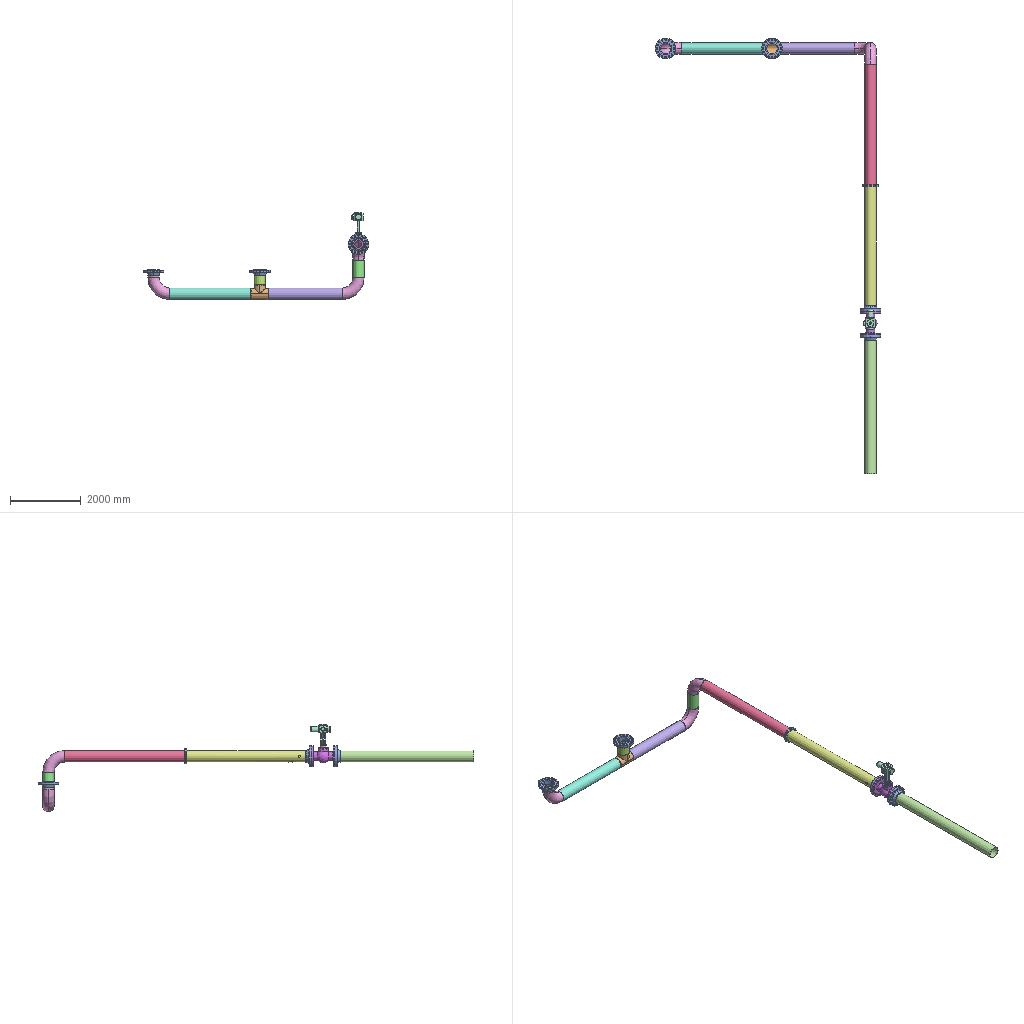Assembly | NX | 16 different items | 22 placed | box 6356 x 12301 x 2462 mm
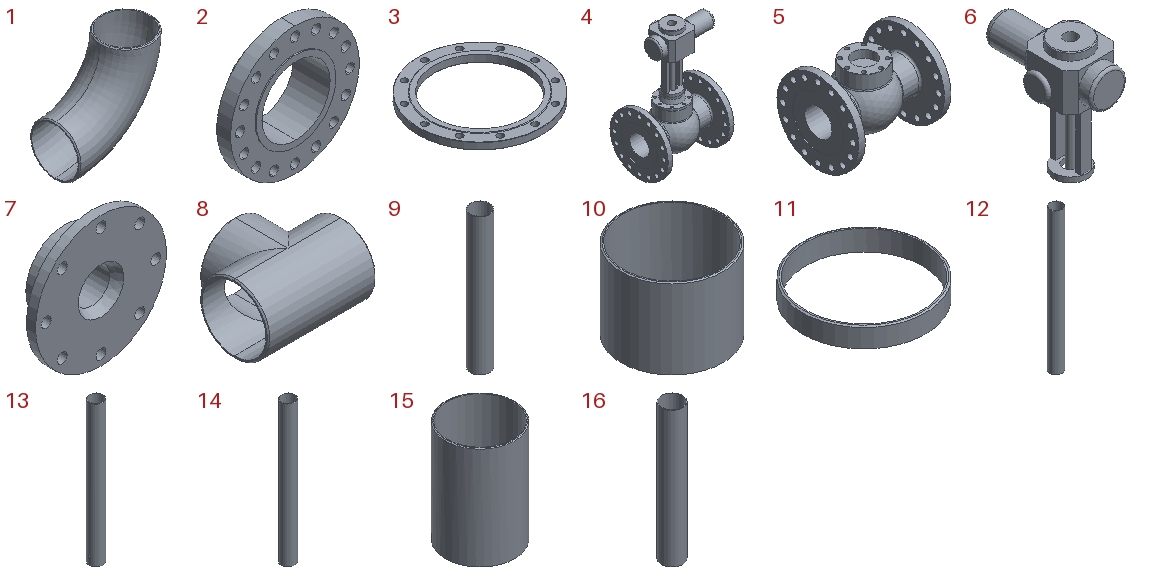Parts list (item | quantity | parent item | size | volume | features):
1 | x3 | - | 619.473 x 325 x 619.47 mm | 8769531 mm3 | features BREP 1
2 | x4 | - | 585 x 167.113 x 585 mm | 13392548 mm3 | features BREP 1, Resize Face 1
3 | x2 | - | 440 x 440 x 26 mm | 1570875 mm3 | features INSTANCE 12, ABSOLUTE_DATUM_PLANE 3, CHAMFER 3, SIMPLE HOLE 2, ABSOLUTE_DATUM_AXIS 1, BOSS 1, CIRCULAR_ISET 1, CYLINDER 1, TRANSFORM_ISET 1
4 | x1 | - | 694.2 x 585 x 1192 mm | 71467012 mm3 | features SKETCH 46, DATUM_CSYS 45, EXTRACT_DATUM_AXIS 40, EXTRACT_FACE 40, HOLE PACKAGE 40, SIMPLE HOLE 40, Instance Feature 22, ABSOLUTE_DATUM_PLANE 11, ABSOLUTE_DATUM_AXIS 7, Resize Face 6, EXTRUDE 3, BREP 2, CPROJ 2, Pattern Feature 2, SWP104 2, AXIS_ANGLE_DATUM_PLANE 1, BLEND 1
5 | x1 | in 4 | 660.4 x 585 x 585 mm | 47612449 mm3 | features SKETCH 35, DATUM_CSYS 34, EXTRACT_DATUM_AXIS 32, EXTRACT_FACE 32, HOLE PACKAGE 32, SIMPLE HOLE 32, Instance Feature 15, ABSOLUTE_DATUM_AXIS 5, ABSOLUTE_DATUM_PLANE 5, Resize Face 3, EXTRUDE 2, AXIS_ANGLE_DATUM_PLANE 1, BREP 1, Pattern Feature 1
6 | x1 | in 4 | 312 x 559 x 624 mm | 21569285 mm3 | features ABSOLUTE_DATUM_PLANE 3, ABSOLUTE_DATUM_AXIS 1, BREP 1
7 | x1 | in 4 | 286 x 80 x 286 mm | 2285168 mm3 | features DATUM_CSYS 11, SKETCH 11, EXTRACT_DATUM_AXIS 8, EXTRACT_FACE 8, HOLE PACKAGE 8, SIMPLE HOLE 8, Instance Feature 7, ABSOLUTE_DATUM_PLANE 3, Resize Face 3, CPROJ 2, SWP104 2, ABSOLUTE_DATUM_AXIS 1, BLEND 1, EXTRUDE 1, Pattern Feature 1
8 | x1 | - | 508 x 416.5 x 325 mm | 6849380 mm3 | features BREP 1
9 | x1 | - | 325 x 325 x 2289 mm | 18225689 mm3 | features CHAMFER 1, CYLINDER 1, DATUM_CSYS 1, SHELL 1
10 | x1 | - | 325 x 325 x 256.774 mm | 2034780 mm3 | features CHAMFER 1, CYLINDER 1, DATUM_CSYS 1, SHELL 1
11 | x1 | - | 325 x 325 x 53.774 mm | 417463 mm3 | features CHAMFER 1, CYLINDER 1, DATUM_CSYS 1, SHELL 1
12 | x1 | - | 325 x 325 x 3759 mm | 29937295 mm3 | features CHAMFER 1, CYLINDER 1, DATUM_CSYS 1, SHELL 1
13 | x1 | - | 325 x 325 x 3360 mm | 26652772 mm3 | features DATUM_CSYS 3, EXTRUDE 2, SKETCH 2, CHAMFER 1, CYLINDER 1, SHELL 1
14 | x1 | - | 325 x 325 x 3398 mm | 27057214 mm3 | features CHAMFER 1, CYLINDER 1, DATUM_CSYS 1, SHELL 1
15 | x1 | - | 325 x 325 x 486 mm | 3861046 mm3 | features CHAMFER 1, CYLINDER 1, DATUM_CSYS 1, SHELL 1
16 | x1 | - | 325 x 325 x 2069 mm | 16472932 mm3 | features CHAMFER 1, CYLINDER 1, DATUM_CSYS 1, SHELL 1
Mates (type | each side: item.copy, entity, surface, feature):
In the top assembly
Fix | 12.1 component
Concentric | 12.1 edge | 2.1 edge
Concentric | 2.1 edge | 5.1 edge
Concentric | 5.1 edge | 2.1 edge
Concentric | 2.1 edge | 13.1 edge
Concentric | 13.1 edge | 3.1 edge
Concentric | 3.1 edge | 3.1 edge
Concentric | 3.1 edge | 14.1 edge
Concentric | 14.1 edge | 1.1 edge
Concentric | 1.1 edge | 15.1 edge | 2 times
Concentric | 1.1 edge | 16.1 edge
Concentric | 16.1 edge | 8.1 edge
Concentric | 8.1 edge | 9.1 edge
Concentric | 9.1 edge | 1.1 edge
Concentric | 10.1 edge | 8.1 edge
Concentric | 10.1 edge | 2.1 edge
Concentric | 1.1 edge | 11.1 edge
Concentric | 2.1 edge | 11.1 edge
In subassembly 4
Fix | 5.1 component
Touch | 7.1 | 5.1 | 2 times
Touch | 6.1 | 7.1
Parallel | 6.1 | 5.1